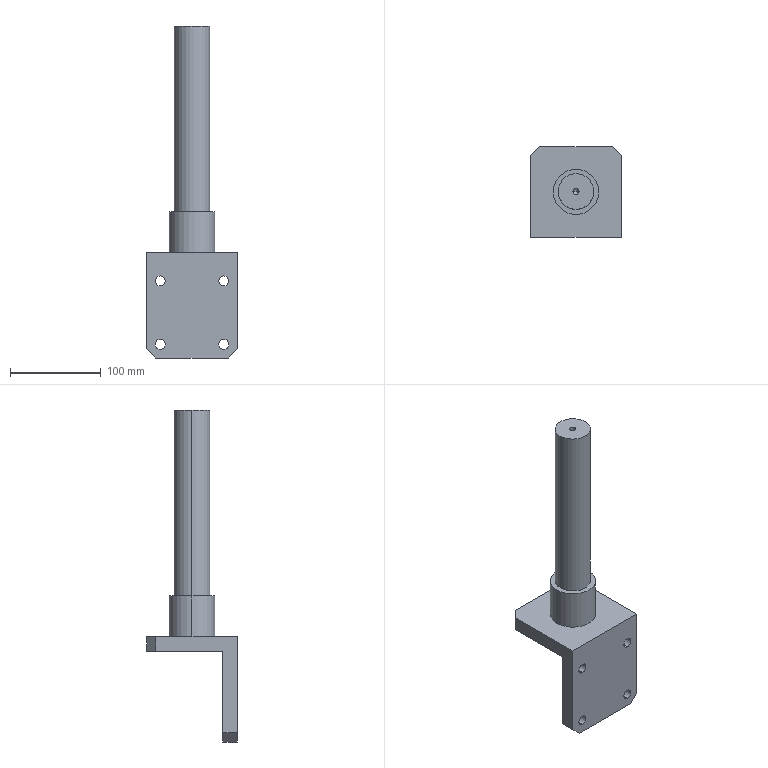Part | SolidWorks | features ICE 3, HoleWzd 2, Chamfer 1, Extrusion 1 | 1 solid | 30 faces | box 100 x 100 x 366 mm | volume 643224 mm3 | cylinder 14 | plane 14 | cone 2 | commonest cylinder face diameters 11 x8 6.8 x2 39 x2 50 x2
STEP:
#1=CARTESIAN_POINT('',(-35.,-50.,-90.5));
#2=VERTEX_POINT('',#1);
#3=CARTESIAN_POINT('',(-35.,-50.,-79.5));
#4=VERTEX_POINT('',#3);
#5=CARTESIAN_POINT('',(-35.,-50.,-85.));
#6=DIRECTION('',(0.,1.,0.));
#7=DIRECTION('',(0.,0.,1.));
#8=AXIS2_PLACEMENT_3D('',#5,#6,#7);
#9=CIRCLE('',#8,5.5);
#10=EDGE_CURVE('',#2,#4,#9,.T.);
#11=ORIENTED_EDGE('',*,*,#10,.F.);
#12=CARTESIAN_POINT('',(-35.,-34.,-90.5));
#13=VERTEX_POINT('',#12);
#14=CARTESIAN_POINT('',(-35.,-34.,-90.5));
#15=DIRECTION('',(0.,1.,0.));
#16=VECTOR('',#15,1000.);
#17=LINE('',#14,#16);
#18=EDGE_CURVE('',#2,#13,#17,.T.);
#19=ORIENTED_EDGE('',*,*,#18,.T.);
#20=CARTESIAN_POINT('',(-35.,-34.,-79.5));
#21=VERTEX_POINT('',#20);
#22=CARTESIAN_POINT('',(-35.,-34.,-85.));
#23=DIRECTION('',(0.,1.,0.));
#24=DIRECTION('',(0.,0.,1.));
#25=AXIS2_PLACEMENT_3D('',#22,#23,#24);
#26=CIRCLE('',#25,5.5);
#27=EDGE_CURVE('',#13,#21,#26,.T.);
#28=ORIENTED_EDGE('',*,*,#27,.T.);
#29=CARTESIAN_POINT('',(-35.,-34.,-79.5));
#30=DIRECTION('',(0.,1.,0.));
#31=VECTOR('',#30,1000.);
#32=LINE('',#29,#31);
#33=EDGE_CURVE('',#4,#21,#32,.T.);
#34=ORIENTED_EDGE('',*,*,#33,.F.);
#35=EDGE_LOOP('',(#11,#19,#28,#34));
#36=FACE_OUTER_BOUND('',#35,.T.);
#37=CARTESIAN_POINT('',(-35.,-34.,-85.));
#38=DIRECTION('',(0.,1.,0.));
#39=DIRECTION('',(0.,0.,1.));
#40=AXIS2_PLACEMENT_3D('',#37,#38,#39);
#41=CYLINDRICAL_SURFACE('',#40,5.5);
#42=ADVANCED_FACE('',(#36),#41,.F.);
#43=CARTESIAN_POINT('',(35.,-50.,-90.5));
#44=VERTEX_POINT('',#43);
#45=CARTESIAN_POINT('',(35.,-50.,-79.5));
#46=VERTEX_POINT('',#45);
#47=CARTESIAN_POINT('',(35.,-50.,-85.));
#48=DIRECTION('',(0.,1.,0.));
#49=DIRECTION('',(0.,0.,1.));
#50=AXIS2_PLACEMENT_3D('',#47,#48,#49);
#51=CIRCLE('',#50,5.5);
#52=EDGE_CURVE('',#44,#46,#51,.T.);
#53=ORIENTED_EDGE('',*,*,#52,.F.);
#54=CARTESIAN_POINT('',(35.,-34.,-90.5));
#55=VERTEX_POINT('',#54);
#56=CARTESIAN_POINT('',(35.,-34.,-90.5));
#57=DIRECTION('',(0.,1.,0.));
#58=VECTOR('',#57,1000.);
#59=LINE('',#56,#58);
#60=EDGE_CURVE('',#44,#55,#59,.T.);
#61=ORIENTED_EDGE('',*,*,#60,.T.);
#62=CARTESIAN_POINT('',(35.,-34.,-79.5));
#63=VERTEX_POINT('',#62);
#64=CARTESIAN_POINT('',(35.,-34.,-85.));
#65=DIRECTION('',(0.,1.,0.));
#66=DIRECTION('',(0.,0.,1.));
#67=AXIS2_PLACEMENT_3D('',#64,#65,#66);
#68=CIRCLE('',#67,5.5);
#69=EDGE_CURVE('',#55,#63,#68,.T.);
#70=ORIENTED_EDGE('',*,*,#69,.T.);
#71=CARTESIAN_POINT('',(35.,-34.,-79.5));
#72=DIRECTION('',(0.,1.,0.));
#73=VECTOR('',#72,1000.);
#74=LINE('',#71,#73);
#75=EDGE_CURVE('',#46,#63,#74,.T.);
#76=ORIENTED_EDGE('',*,*,#75,.F.);
#77=EDGE_LOOP('',(#53,#61,#70,#76));
#78=FACE_OUTER_BOUND('',#77,.T.);
#79=CARTESIAN_POINT('',(35.,-34.,-85.));
#80=DIRECTION('',(0.,1.,0.));
#81=DIRECTION('',(0.,0.,1.));
#82=AXIS2_PLACEMENT_3D('',#79,#80,#81);
#83=CYLINDRICAL_SURFACE('',#82,5.5);
#84=ADVANCED_FACE('',(#78),#83,.F.);
#85=CARTESIAN_POINT('',(35.,-50.,-20.5));
#86=VERTEX_POINT('',#85);
#87=CARTESIAN_POINT('',(35.,-50.,-9.5));
#88=VERTEX_POINT('',#87);
#89=CARTESIAN_POINT('',(35.,-50.,-15.));
#90=DIRECTION('',(0.,1.,0.));
#91=DIRECTION('',(0.,0.,1.));
#92=AXIS2_PLACEMENT_3D('',#89,#90,#91);
#93=CIRCLE('',#92,5.5);
#94=EDGE_CURVE('',#86,#88,#93,.T.);
#95=ORIENTED_EDGE('',*,*,#94,.F.);
#96=CARTESIAN_POINT('',(35.,-34.,-20.5));
#97=VERTEX_POINT('',#96);
#98=CARTESIAN_POINT('',(35.,-34.,-20.5));
#99=DIRECTION('',(0.,1.,0.));
#100=VECTOR('',#99,1000.);
#101=LINE('',#98,#100);
#102=EDGE_CURVE('',#86,#97,#101,.T.);
#103=ORIENTED_EDGE('',*,*,#102,.T.);
#104=CARTESIAN_POINT('',(35.,-34.,-9.5));
#105=VERTEX_POINT('',#104);
#106=CARTESIAN_POINT('',(35.,-34.,-15.));
#107=DIRECTION('',(0.,1.,0.));
#108=DIRECTION('',(0.,0.,1.));
#109=AXIS2_PLACEMENT_3D('',#106,#107,#108);
#110=CIRCLE('',#109,5.5);
#111=EDGE_CURVE('',#97,#105,#110,.T.);
#112=ORIENTED_EDGE('',*,*,#111,.T.);
#113=CARTESIAN_POINT('',(35.,-34.,-9.5));
#114=DIRECTION('',(0.,1.,0.));
#115=VECTOR('',#114,1000.);
#116=LINE('',#113,#115);
#117=EDGE_CURVE('',#88,#105,#116,.T.);
#118=ORIENTED_EDGE('',*,*,#117,.F.);
#119=EDGE_LOOP('',(#95,#103,#112,#118));
#120=FACE_OUTER_BOUND('',#119,.T.);
#121=CARTESIAN_POINT('',(35.,-34.,-15.));
#122=DIRECTION('',(0.,1.,0.));
#123=DIRECTION('',(0.,0.,1.));
#124=AXIS2_PLACEMENT_3D('',#121,#122,#123);
#125=CYLINDRICAL_SURFACE('',#124,5.5);
#126=ADVANCED_FACE('',(#120),#125,.F.);
#127=CARTESIAN_POINT('',(-35.,-50.,-20.5));
#128=VERTEX_POINT('',#127);
#129=CARTESIAN_POINT('',(-35.,-50.,-9.5));
#130=VERTEX_POINT('',#129);
#131=CARTESIAN_POINT('',(-35.,-50.,-15.));
#132=DIRECTION('',(0.,1.,0.));
#133=DIRECTION('',(0.,0.,1.));
#134=AXIS2_PLACEMENT_3D('',#131,#132,#133);
#135=CIRCLE('',#134,5.5);
#136=EDGE_CURVE('',#128,#130,#135,.T.);
#137=ORIENTED_EDGE('',*,*,#136,.F.);
#138=CARTESIAN_POINT('',(-35.,-34.,-20.5));
#139=VERTEX_POINT('',#138);
#140=CARTESIAN_POINT('',(-35.,-34.,-20.5));
#141=DIRECTION('',(0.,1.,0.));
#142=VECTOR('',#141,1000.);
#143=LINE('',#140,#142);
#144=EDGE_CURVE('',#128,#139,#143,.T.);
#145=ORIENTED_EDGE('',*,*,#144,.T.);
#146=CARTESIAN_POINT('',(-35.,-34.,-9.5));
#147=VERTEX_POINT('',#146);
#148=CARTESIAN_POINT('',(-35.,-34.,-15.));
#149=DIRECTION('',(0.,1.,0.));
#150=DIRECTION('',(0.,0.,1.));
#151=AXIS2_PLACEMENT_3D('',#148,#149,#150);
#152=CIRCLE('',#151,5.5);
#153=EDGE_CURVE('',#139,#147,#152,.T.);
#154=ORIENTED_EDGE('',*,*,#153,.T.);
#155=CARTESIAN_POINT('',(-35.,-34.,-9.5));
#156=DIRECTION('',(0.,1.,0.));
#157=VECTOR('',#156,1000.);
#158=LINE('',#155,#157);
#159=EDGE_CURVE('',#130,#147,#158,.T.);
#160=ORIENTED_EDGE('',*,*,#159,.F.);
#161=EDGE_LOOP('',(#137,#145,#154,#160));
#162=FACE_OUTER_BOUND('',#161,.T.);
#163=CARTESIAN_POINT('',(-35.,-34.,-15.));
#164=DIRECTION('',(0.,1.,0.));
#165=DIRECTION('',(0.,0.,1.));
#166=AXIS2_PLACEMENT_3D('',#163,#164,#165);
#167=CYLINDRICAL_SURFACE('',#166,5.5);
#168=ADVANCED_FACE('',(#162),#167,.F.);
#169=CARTESIAN_POINT('',(-3.4,0.,246.25));
#170=VERTEX_POINT('',#169);
#171=CARTESIAN_POINT('',(3.4,0.,246.25));
#172=VERTEX_POINT('',#171);
#173=CARTESIAN_POINT('',(0.,0.,246.25));
#174=DIRECTION('',(0.,0.,1.));
#175=DIRECTION('',(1.,0.,0.));
#176=AXIS2_PLACEMENT_3D('',#173,#174,#175);
#177=CIRCLE('',#176,3.4);
#178=EDGE_CURVE('',#170,#172,#177,.T.);
#179=ORIENTED_EDGE('',*,*,#178,.F.);
#180=CARTESIAN_POINT('',(-3.4,0.,266.));
#181=VERTEX_POINT('',#180);
#182=CARTESIAN_POINT('',(-3.4,0.,266.));
#183=DIRECTION('',(0.,0.,1.));
#184=VECTOR('',#183,1000.);
#185=LINE('',#182,#184);
#186=EDGE_CURVE('',#170,#181,#185,.T.);
#187=ORIENTED_EDGE('',*,*,#186,.T.);
#188=CARTESIAN_POINT('',(3.4,0.,266.));
#189=VERTEX_POINT('',#188);
#190=CARTESIAN_POINT('',(0.,0.,266.));
#191=DIRECTION('',(0.,0.,1.));
#192=DIRECTION('',(1.,0.,0.));
#193=AXIS2_PLACEMENT_3D('',#190,#191,#192);
#194=CIRCLE('',#193,3.4);
#195=EDGE_CURVE('',#181,#189,#194,.T.);
#196=ORIENTED_EDGE('',*,*,#195,.T.);
#197=CARTESIAN_POINT('',(3.4,0.,266.));
#198=DIRECTION('',(0.,0.,1.));
#199=VECTOR('',#198,1000.);
#200=LINE('',#197,#199);
#201=EDGE_CURVE('',#172,#189,#200,.T.);
#202=ORIENTED_EDGE('',*,*,#201,.F.);
#203=EDGE_LOOP('',(#179,#187,#196,#202));
#204=FACE_OUTER_BOUND('',#203,.T.);
#205=CARTESIAN_POINT('',(0.,0.,266.));
#206=DIRECTION('',(0.,0.,1.));
#207=DIRECTION('',(1.,0.,0.));
#208=AXIS2_PLACEMENT_3D('',#205,#206,#207);
#209=CYLINDRICAL_SURFACE('',#208,3.4);
#210=ADVANCED_FACE('',(#204),#209,.F.);
#211=CARTESIAN_POINT('',(0.,0.,244.207));
#212=VERTEX_POINT('',#211);
#213=CARTESIAN_POINT('',(3.4,0.,246.25));
#214=DIRECTION('',(0.8572,0.,0.515));
#215=VECTOR('',#214,1000.);
#216=LINE('',#213,#215);
#217=EDGE_CURVE('',#212,#172,#216,.T.);
#218=ORIENTED_EDGE('',*,*,#217,.F.);
#219=CARTESIAN_POINT('',(-3.4,0.,246.25));
#220=DIRECTION('',(-0.8572,0.,0.515));
#221=VECTOR('',#220,1000.);
#222=LINE('',#219,#221);
#223=EDGE_CURVE('',#212,#170,#222,.T.);
#224=ORIENTED_EDGE('',*,*,#223,.T.);
#225=ORIENTED_EDGE('',*,*,#178,.T.);
#226=EDGE_LOOP('',(#218,#224,#225));
#227=FACE_OUTER_BOUND('',#226,.T.);
#228=CARTESIAN_POINT('',(0.,0.,246.25));
#229=DIRECTION('',(0.,0.,1.));
#230=DIRECTION('',(1.,0.,0.));
#231=AXIS2_PLACEMENT_3D('',#228,#229,#230);
#232=CONICAL_SURFACE('',#231,3.4,1.03);
#233=ADVANCED_FACE('',(#227),#232,.F.);
#234=CARTESIAN_POINT('',(19.5,0.,61.));
#235=VERTEX_POINT('',#234);
#236=CARTESIAN_POINT('',(-19.5,0.,61.));
#237=VERTEX_POINT('',#236);
#238=CARTESIAN_POINT('',(0.,0.,61.));
#239=DIRECTION('',(0.,0.,1.));
#240=DIRECTION('',(1.,0.,0.));
#241=AXIS2_PLACEMENT_3D('',#238,#239,#240);
#242=CIRCLE('',#241,19.5);
#243=EDGE_CURVE('',#235,#237,#242,.T.);
#244=ORIENTED_EDGE('',*,*,#243,.T.);
#245=CARTESIAN_POINT('',(-19.5,0.,266.));
#246=VERTEX_POINT('',#245);
#247=CARTESIAN_POINT('',(-19.5,0.,61.));
#248=DIRECTION('',(0.,0.,1.));
#249=VECTOR('',#248,1000.);
#250=LINE('',#247,#249);
#251=EDGE_CURVE('',#237,#246,#250,.T.);
#252=ORIENTED_EDGE('',*,*,#251,.T.);
#253=CARTESIAN_POINT('',(19.5,0.,266.));
#254=VERTEX_POINT('',#253);
#255=CARTESIAN_POINT('',(0.,0.,266.));
#256=DIRECTION('',(0.,0.,1.));
#257=DIRECTION('',(1.,0.,0.));
#258=AXIS2_PLACEMENT_3D('',#255,#256,#257);
#259=CIRCLE('',#258,19.5);
#260=EDGE_CURVE('',#254,#246,#259,.T.);
#261=ORIENTED_EDGE('',*,*,#260,.F.);
#262=CARTESIAN_POINT('',(19.5,0.,61.));
#263=DIRECTION('',(0.,0.,1.));
#264=VECTOR('',#263,1000.);
#265=LINE('',#262,#264);
#266=EDGE_CURVE('',#235,#254,#265,.T.);
#267=ORIENTED_EDGE('',*,*,#266,.F.);
#268=EDGE_LOOP('',(#244,#252,#261,#267));
#269=FACE_OUTER_BOUND('',#268,.T.);
#270=CARTESIAN_POINT('',(0.,0.,61.));
#271=DIRECTION('',(0.,0.,1.));
#272=DIRECTION('',(1.,0.,0.));
#273=AXIS2_PLACEMENT_3D('',#270,#271,#272);
#274=CYLINDRICAL_SURFACE('',#273,19.5);
#275=ADVANCED_FACE('',(#269),#274,.T.);
#276=CARTESIAN_POINT('',(25.,0.,61.));
#277=VERTEX_POINT('',#276);
#278=CARTESIAN_POINT('',(-25.,0.,61.));
#279=VERTEX_POINT('',#278);
#280=CARTESIAN_POINT('',(0.,0.,61.));
#281=DIRECTION('',(0.,0.,1.));
#282=DIRECTION('',(1.,0.,0.));
#283=AXIS2_PLACEMENT_3D('',#280,#281,#282);
#284=CIRCLE('',#283,25.);
#285=EDGE_CURVE('',#277,#279,#284,.T.);
#286=ORIENTED_EDGE('',*,*,#285,.F.);
#287=CARTESIAN_POINT('',(25.,0.,16.));
#288=VERTEX_POINT('',#287);
#289=CARTESIAN_POINT('',(25.,0.,266.));
#290=DIRECTION('',(0.,0.,-1.));
#291=VECTOR('',#290,1000.);
#292=LINE('',#289,#291);
#293=EDGE_CURVE('',#277,#288,#292,.T.);
#294=ORIENTED_EDGE('',*,*,#293,.T.);
#295=CARTESIAN_POINT('',(-25.,0.,16.));
#296=VERTEX_POINT('',#295);
#297=CARTESIAN_POINT('',(0.,0.,16.));
#298=DIRECTION('',(0.,0.,1.));
#299=DIRECTION('',(1.,0.,0.));
#300=AXIS2_PLACEMENT_3D('',#297,#298,#299);
#301=CIRCLE('',#300,25.);
#302=EDGE_CURVE('',#288,#296,#301,.T.);
#303=ORIENTED_EDGE('',*,*,#302,.T.);
#304=CARTESIAN_POINT('',(-25.,0.,266.));
#305=DIRECTION('',(0.,0.,-1.));
#306=VECTOR('',#305,1000.);
#307=LINE('',#304,#306);
#308=EDGE_CURVE('',#279,#296,#307,.T.);
#309=ORIENTED_EDGE('',*,*,#308,.F.);
#310=EDGE_LOOP('',(#286,#294,#303,#309));
#311=FACE_OUTER_BOUND('',#310,.T.);
#312=CARTESIAN_POINT('',(0.,0.,266.));
#313=DIRECTION('',(0.,0.,-1.));
#314=DIRECTION('',(-1.,0.,0.));
#315=AXIS2_PLACEMENT_3D('',#312,#313,#314);
#316=CYLINDRICAL_SURFACE('',#315,25.);
#317=ADVANCED_FACE('',(#311),#316,.T.);
#318=CARTESIAN_POINT('',(-35.,-34.,-85.));
#319=DIRECTION('',(0.,1.,0.));
#320=DIRECTION('',(0.,0.,1.));
#321=AXIS2_PLACEMENT_3D('',#318,#319,#320);
#322=CIRCLE('',#321,5.5);
#323=EDGE_CURVE('',#21,#13,#322,.T.);
#324=ORIENTED_EDGE('',*,*,#323,.F.);
#325=ORIENTED_EDGE('',*,*,#27,.F.);
#326=EDGE_LOOP('',(#324,#325));
#327=FACE_BOUND('',#326,.T.);
#328=CARTESIAN_POINT('',(35.,-34.,-85.));
#329=DIRECTION('',(0.,1.,0.));
#330=DIRECTION('',(0.,0.,1.));
#331=AXIS2_PLACEMENT_3D('',#328,#329,#330);
#332=CIRCLE('',#331,5.5);
#333=EDGE_CURVE('',#63,#55,#332,.T.);
#334=ORIENTED_EDGE('',*,*,#333,.F.);
#335=ORIENTED_EDGE('',*,*,#69,.F.);
#336=EDGE_LOOP('',(#334,#335));
#337=FACE_BOUND('',#336,.T.);
#338=CARTESIAN_POINT('',(35.,-34.,-15.));
#339=DIRECTION('',(0.,1.,0.));
#340=DIRECTION('',(0.,0.,1.));
#341=AXIS2_PLACEMENT_3D('',#338,#339,#340);
#342=CIRCLE('',#341,5.5);
#343=EDGE_CURVE('',#105,#97,#342,.T.);
#344=ORIENTED_EDGE('',*,*,#343,.F.);
#345=ORIENTED_EDGE('',*,*,#111,.F.);
#346=EDGE_LOOP('',(#344,#345));
#347=FACE_BOUND('',#346,.T.);
#348=CARTESIAN_POINT('',(-40.,-34.,-100.));
#349=VERTEX_POINT('',#348);
#350=CARTESIAN_POINT('',(40.,-34.,-100.));
#351=VERTEX_POINT('',#350);
#352=CARTESIAN_POINT('',(-50.,-34.,-100.));
#353=DIRECTION('',(1.,0.,0.));
#354=VECTOR('',#353,1000.);
#355=LINE('',#352,#354);
#356=EDGE_CURVE('',#349,#351,#355,.T.);
#357=ORIENTED_EDGE('',*,*,#356,.F.);
#358=CARTESIAN_POINT('',(-50.,-34.,-90.));
#359=VERTEX_POINT('',#358);
#360=CARTESIAN_POINT('',(-40.,-34.,-100.));
#361=DIRECTION('',(-0.7071,0.,0.7071));
#362=VECTOR('',#361,1000.);
#363=LINE('',#360,#362);
#364=EDGE_CURVE('',#349,#359,#363,.T.);
#365=ORIENTED_EDGE('',*,*,#364,.T.);
#366=CARTESIAN_POINT('',(-50.,-34.,0.));
#367=VERTEX_POINT('',#366);
#368=CARTESIAN_POINT('',(-50.,-34.,-100.));
#369=DIRECTION('',(0.,0.,1.));
#370=VECTOR('',#369,1000.);
#371=LINE('',#368,#370);
#372=EDGE_CURVE('',#359,#367,#371,.T.);
#373=ORIENTED_EDGE('',*,*,#372,.T.);
#374=CARTESIAN_POINT('',(50.,-34.,0.));
#375=VERTEX_POINT('',#374);
#376=CARTESIAN_POINT('',(-50.,-34.,0.));
#377=DIRECTION('',(1.,0.,0.));
#378=VECTOR('',#377,1000.);
#379=LINE('',#376,#378);
#380=EDGE_CURVE('',#367,#375,#379,.T.);
#381=ORIENTED_EDGE('',*,*,#380,.T.);
#382=CARTESIAN_POINT('',(50.,-34.,-90.));
#383=VERTEX_POINT('',#382);
#384=CARTESIAN_POINT('',(50.,-34.,-100.));
#385=DIRECTION('',(0.,0.,1.));
#386=VECTOR('',#385,1000.);
#387=LINE('',#384,#386);
#388=EDGE_CURVE('',#383,#375,#387,.T.);
#389=ORIENTED_EDGE('',*,*,#388,.F.);
#390=CARTESIAN_POINT('',(40.,-34.,-100.));
#391=DIRECTION('',(-0.7071,0.,-0.7071));
#392=VECTOR('',#391,1000.);
#393=LINE('',#390,#392);
#394=EDGE_CURVE('',#383,#351,#393,.T.);
#395=ORIENTED_EDGE('',*,*,#394,.T.);
#396=EDGE_LOOP('',(#357,#365,#373,#381,#389,#395));
#397=FACE_OUTER_BOUND('',#396,.T.);
#398=CARTESIAN_POINT('',(-35.,-34.,-15.));
#399=DIRECTION('',(0.,1.,0.));
#400=DIRECTION('',(0.,0.,1.));
#401=AXIS2_PLACEMENT_3D('',#398,#399,#400);
#402=CIRCLE('',#401,5.5);
#403=EDGE_CURVE('',#147,#139,#402,.T.);
#404=ORIENTED_EDGE('',*,*,#403,.F.);
#405=ORIENTED_EDGE('',*,*,#153,.F.);
#406=EDGE_LOOP('',(#404,#405));
#407=FACE_BOUND('',#406,.T.);
#408=CARTESIAN_POINT('',(-50.,-34.,-100.));
#409=DIRECTION('',(0.,-1.,0.));
#410=DIRECTION('',(1.,0.,0.));
#411=AXIS2_PLACEMENT_3D('',#408,#409,#410);
#412=PLANE('',#411);
#413=ADVANCED_FACE('',(#327,#337,#347,#397,#407),#412,.F.);
#414=ORIENTED_EDGE('',*,*,#293,.F.);
#415=CARTESIAN_POINT('',(0.,0.,61.));
#416=DIRECTION('',(0.,0.,1.));
#417=DIRECTION('',(1.,0.,0.));
#418=AXIS2_PLACEMENT_3D('',#415,#416,#417);
#419=CIRCLE('',#418,25.);
#420=EDGE_CURVE('',#279,#277,#419,.T.);
#421=ORIENTED_EDGE('',*,*,#420,.F.);
#422=ORIENTED_EDGE('',*,*,#308,.T.);
#423=CARTESIAN_POINT('',(0.,0.,16.));
#424=DIRECTION('',(0.,0.,1.));
#425=DIRECTION('',(1.,0.,0.));
#426=AXIS2_PLACEMENT_3D('',#423,#424,#425);
#427=CIRCLE('',#426,25.);
#428=EDGE_CURVE('',#296,#288,#427,.T.);
#429=ORIENTED_EDGE('',*,*,#428,.T.);
#430=EDGE_LOOP('',(#414,#421,#422,#429));
#431=FACE_OUTER_BOUND('',#430,.T.);
#432=CARTESIAN_POINT('',(0.,0.,266.));
#433=DIRECTION('',(0.,0.,-1.));
#434=DIRECTION('',(-1.,0.,0.));
#435=AXIS2_PLACEMENT_3D('',#432,#433,#434);
#436=CYLINDRICAL_SURFACE('',#435,25.);
#437=ADVANCED_FACE('',(#431),#436,.T.);
#438=CARTESIAN_POINT('',(50.,-50.,16.));
#439=VERTEX_POINT('',#438);
#440=CARTESIAN_POINT('',(50.,-50.,-90.));
#441=VERTEX_POINT('',#440);
#442=CARTESIAN_POINT('',(50.,-50.,16.));
#443=DIRECTION('',(0.,0.,-1.));
#444=VECTOR('',#443,1000.);
#445=LINE('',#442,#444);
#446=EDGE_CURVE('',#439,#441,#445,.T.);
#447=ORIENTED_EDGE('',*,*,#446,.T.);
#448=CARTESIAN_POINT('',(50.,-34.,-90.));
#449=DIRECTION('',(0.,1.,0.));
#450=VECTOR('',#449,1000.);
#451=LINE('',#448,#450);
#452=EDGE_CURVE('',#441,#383,#451,.T.);
#453=ORIENTED_EDGE('',*,*,#452,.T.);
#454=ORIENTED_EDGE('',*,*,#388,.T.);
#455=CARTESIAN_POINT('',(50.,40.,0.));
#456=VERTEX_POINT('',#455);
#457=CARTESIAN_POINT('',(50.,-50.,0.));
#458=DIRECTION('',(0.,1.,0.));
#459=VECTOR('',#458,1000.);
#460=LINE('',#457,#459);
#461=EDGE_CURVE('',#375,#456,#460,.T.);
#462=ORIENTED_EDGE('',*,*,#461,.T.);
#463=CARTESIAN_POINT('',(50.,40.,16.));
#464=VERTEX_POINT('',#463);
#465=CARTESIAN_POINT('',(50.,40.,16.));
#466=DIRECTION('',(0.,0.,1.));
#467=VECTOR('',#466,1000.);
#468=LINE('',#465,#467);
#469=EDGE_CURVE('',#456,#464,#468,.T.);
#470=ORIENTED_EDGE('',*,*,#469,.T.);
#471=CARTESIAN_POINT('',(50.,-50.,16.));
#472=DIRECTION('',(0.,1.,0.));
#473=VECTOR('',#472,1000.);
#474=LINE('',#471,#473);
#475=EDGE_CURVE('',#439,#464,#474,.T.);
#476=ORIENTED_EDGE('',*,*,#475,.F.);
#477=EDGE_LOOP('',(#447,#453,#454,#462,#470,#476));
#478=FACE_OUTER_BOUND('',#477,.T.);
#479=CARTESIAN_POINT('',(50.,-50.,16.));
#480=DIRECTION('',(-1.,0.,0.));
#481=DIRECTION('',(0.,0.,1.));
#482=AXIS2_PLACEMENT_3D('',#479,#480,#481);
#483=PLANE('',#482);
#484=ADVANCED_FACE('',(#478),#483,.F.);
#485=CARTESIAN_POINT('',(40.,50.,16.));
#486=VERTEX_POINT('',#485);
#487=CARTESIAN_POINT('',(-40.,50.,16.));
#488=VERTEX_POINT('',#487);
#489=CARTESIAN_POINT('',(-50.,50.,16.));
#490=DIRECTION('',(-1.,0.,0.));
#491=VECTOR('',#490,1000.);
#492=LINE('',#489,#491);
#493=EDGE_CURVE('',#486,#488,#492,.T.);
#494=ORIENTED_EDGE('',*,*,#493,.F.);
#495=CARTESIAN_POINT('',(40.,50.,0.));
#496=VERTEX_POINT('',#495);
#497=CARTESIAN_POINT('',(40.,50.,16.));
#498=DIRECTION('',(0.,0.,-1.));
#499=VECTOR('',#498,1000.);
#500=LINE('',#497,#499);
#501=EDGE_CURVE('',#486,#496,#500,.T.);
#502=ORIENTED_EDGE('',*,*,#501,.T.);
#503=CARTESIAN_POINT('',(-40.,50.,0.));
#504=VERTEX_POINT('',#503);
#505=CARTESIAN_POINT('',(-50.,50.,0.));
#506=DIRECTION('',(-1.,0.,0.));
#507=VECTOR('',#506,1000.);
#508=LINE('',#505,#507);
#509=EDGE_CURVE('',#496,#504,#508,.T.);
#510=ORIENTED_EDGE('',*,*,#509,.T.);
#511=CARTESIAN_POINT('',(-40.,50.,16.));
#512=DIRECTION('',(0.,0.,1.));
#513=VECTOR('',#512,1000.);
#514=LINE('',#511,#513);
#515=EDGE_CURVE('',#504,#488,#514,.T.);
#516=ORIENTED_EDGE('',*,*,#515,.T.);
#517=EDGE_LOOP('',(#494,#502,#510,#516));
#518=FACE_OUTER_BOUND('',#517,.T.);
#519=CARTESIAN_POINT('',(-50.,50.,16.));
#520=DIRECTION('',(0.,-1.,0.));
#521=DIRECTION('',(0.,0.,-1.));
#522=AXIS2_PLACEMENT_3D('',#519,#520,#521);
#523=PLANE('',#522);
#524=ADVANCED_FACE('',(#518),#523,.F.);
#525=ORIENTED_EDGE('',*,*,#372,.F.);
#526=CARTESIAN_POINT('',(-50.,-50.,-90.));
#527=VERTEX_POINT('',#526);
#528=CARTESIAN_POINT('',(-50.,-50.,-90.));
#529=DIRECTION('',(0.,-1.,0.));
#530=VECTOR('',#529,1000.);
#531=LINE('',#528,#530);
#532=EDGE_CURVE('',#359,#527,#531,.T.);
#533=ORIENTED_EDGE('',*,*,#532,.T.);
#534=CARTESIAN_POINT('',(-50.,-50.,16.));
#535=VERTEX_POINT('',#534);
#536=CARTESIAN_POINT('',(-50.,-50.,16.));
#537=DIRECTION('',(0.,0.,-1.));
#538=VECTOR('',#537,1000.);
#539=LINE('',#536,#538);
#540=EDGE_CURVE('',#535,#527,#539,.T.);
#541=ORIENTED_EDGE('',*,*,#540,.F.);
#542=CARTESIAN_POINT('',(-50.,40.,16.));
#543=VERTEX_POINT('',#542);
#544=CARTESIAN_POINT('',(-50.,-50.,16.));
#545=DIRECTION('',(0.,-1.,0.));
#546=VECTOR('',#545,1000.);
#547=LINE('',#544,#546);
#548=EDGE_CURVE('',#543,#535,#547,.T.);
#549=ORIENTED_EDGE('',*,*,#548,.F.);
#550=CARTESIAN_POINT('',(-50.,40.,0.));
#551=VERTEX_POINT('',#550);
#552=CARTESIAN_POINT('',(-50.,40.,16.));
#553=DIRECTION('',(0.,0.,-1.));
#554=VECTOR('',#553,1000.);
#555=LINE('',#552,#554);
#556=EDGE_CURVE('',#543,#551,#555,.T.);
#557=ORIENTED_EDGE('',*,*,#556,.T.);
#558=CARTESIAN_POINT('',(-50.,-50.,0.));
#559=DIRECTION('',(0.,-1.,0.));
#560=VECTOR('',#559,1000.);
#561=LINE('',#558,#560);
#562=EDGE_CURVE('',#551,#367,#561,.T.);
#563=ORIENTED_EDGE('',*,*,#562,.T.);
#564=EDGE_LOOP('',(#525,#533,#541,#549,#557,#563));
#565=FACE_OUTER_BOUND('',#564,.T.);
#566=CARTESIAN_POINT('',(-50.,-50.,16.));
#567=DIRECTION('',(1.,0.,0.));
#568=DIRECTION('',(0.,0.,-1.));
#569=AXIS2_PLACEMENT_3D('',#566,#567,#568);
#570=PLANE('',#569);
#571=ADVANCED_FACE('',(#565),#570,.F.);
#572=CARTESIAN_POINT('',(-35.,-50.,-85.));
#573=DIRECTION('',(0.,1.,0.));
#574=DIRECTION('',(0.,0.,1.));
#575=AXIS2_PLACEMENT_3D('',#572,#573,#574);
#576=CIRCLE('',#575,5.5);
#577=EDGE_CURVE('',#4,#2,#576,.T.);
#578=ORIENTED_EDGE('',*,*,#577,.T.);
#579=ORIENTED_EDGE('',*,*,#10,.T.);
#580=EDGE_LOOP('',(#578,#579));
#581=FACE_BOUND('',#580,.T.);
#582=CARTESIAN_POINT('',(35.,-50.,-85.));
#583=DIRECTION('',(0.,1.,0.));
#584=DIRECTION('',(0.,0.,1.));
#585=AXIS2_PLACEMENT_3D('',#582,#583,#584);
#586=CIRCLE('',#585,5.5);
#587=EDGE_CURVE('',#46,#44,#586,.T.);
#588=ORIENTED_EDGE('',*,*,#587,.T.);
#589=ORIENTED_EDGE('',*,*,#52,.T.);
#590=EDGE_LOOP('',(#588,#589));
#591=FACE_BOUND('',#590,.T.);
#592=CARTESIAN_POINT('',(35.,-50.,-15.));
#593=DIRECTION('',(0.,1.,0.));
#594=DIRECTION('',(0.,0.,1.));
#595=AXIS2_PLACEMENT_3D('',#592,#593,#594);
#596=CIRCLE('',#595,5.5);
#597=EDGE_CURVE('',#88,#86,#596,.T.);
#598=ORIENTED_EDGE('',*,*,#597,.T.);
#599=ORIENTED_EDGE('',*,*,#94,.T.);
#600=EDGE_LOOP('',(#598,#599));
#601=FACE_BOUND('',#600,.T.);
#602=CARTESIAN_POINT('',(-35.,-50.,-15.));
#603=DIRECTION('',(0.,1.,0.));
#604=DIRECTION('',(0.,0.,1.));
#605=AXIS2_PLACEMENT_3D('',#602,#603,#604);
#606=CIRCLE('',#605,5.5);
#607=EDGE_CURVE('',#130,#128,#606,.T.);
#608=ORIENTED_EDGE('',*,*,#607,.T.);
#609=ORIENTED_EDGE('',*,*,#136,.T.);
#610=EDGE_LOOP('',(#608,#609));
#611=FACE_BOUND('',#610,.T.);
#612=ORIENTED_EDGE('',*,*,#540,.T.);
#613=CARTESIAN_POINT('',(-40.,-50.,-100.));
#614=VERTEX_POINT('',#613);
#615=CARTESIAN_POINT('',(-40.,-50.,-100.));
#616=DIRECTION('',(0.7071,0.,-0.7071));
#617=VECTOR('',#616,1000.);
#618=LINE('',#615,#617);
#619=EDGE_CURVE('',#527,#614,#618,.T.);
#620=ORIENTED_EDGE('',*,*,#619,.T.);
#621=CARTESIAN_POINT('',(40.,-50.,-100.));
#622=VERTEX_POINT('',#621);
#623=CARTESIAN_POINT('',(-50.,-50.,-100.));
#624=DIRECTION('',(-1.,0.,0.));
#625=VECTOR('',#624,1000.);
#626=LINE('',#623,#625);
#627=EDGE_CURVE('',#622,#614,#626,.T.);
#628=ORIENTED_EDGE('',*,*,#627,.F.);
#629=CARTESIAN_POINT('',(40.,-50.,-100.));
#630=DIRECTION('',(0.7071,0.,0.7071));
#631=VECTOR('',#630,1000.);
#632=LINE('',#629,#631);
#633=EDGE_CURVE('',#622,#441,#632,.T.);
#634=ORIENTED_EDGE('',*,*,#633,.T.);
#635=ORIENTED_EDGE('',*,*,#446,.F.);
#636=CARTESIAN_POINT('',(-50.,-50.,16.));
#637=DIRECTION('',(1.,0.,0.));
#638=VECTOR('',#637,1000.);
#639=LINE('',#636,#638);
#640=EDGE_CURVE('',#535,#439,#639,.T.);
#641=ORIENTED_EDGE('',*,*,#640,.F.);
#642=EDGE_LOOP('',(#612,#620,#628,#634,#635,#641));
#643=FACE_OUTER_BOUND('',#642,.T.);
#644=CARTESIAN_POINT('',(-50.,-50.,16.));
#645=DIRECTION('',(0.,1.,0.));
#646=DIRECTION('',(0.,0.,1.));
#647=AXIS2_PLACEMENT_3D('',#644,#645,#646);
#648=PLANE('',#647);
#649=ADVANCED_FACE('',(#581,#591,#601,#611,#643),#648,.F.);
#650=ORIENTED_EDGE('',*,*,#428,.F.);
#651=ORIENTED_EDGE('',*,*,#302,.F.);
#652=EDGE_LOOP('',(#650,#651));
#653=FACE_BOUND('',#652,.T.);
#654=ORIENTED_EDGE('',*,*,#475,.T.);
#655=CARTESIAN_POINT('',(40.,50.,16.));
#656=DIRECTION('',(-0.7071,0.7071,0.));
#657=VECTOR('',#656,1000.);
#658=LINE('',#655,#657);
#659=EDGE_CURVE('',#464,#486,#658,.T.);
#660=ORIENTED_EDGE('',*,*,#659,.T.);
#661=ORIENTED_EDGE('',*,*,#493,.T.);
#662=CARTESIAN_POINT('',(-50.,40.,16.));
#663=DIRECTION('',(-0.7071,-0.7071,0.));
#664=VECTOR('',#663,1000.);
#665=LINE('',#662,#664);
#666=EDGE_CURVE('',#488,#543,#665,.T.);
#667=ORIENTED_EDGE('',*,*,#666,.T.);
#668=ORIENTED_EDGE('',*,*,#548,.T.);
#669=ORIENTED_EDGE('',*,*,#640,.T.);
#670=EDGE_LOOP('',(#654,#660,#661,#667,#668,#669));
#671=FACE_OUTER_BOUND('',#670,.T.);
#672=CARTESIAN_POINT('',(0.,0.,16.));
#673=DIRECTION('',(0.,0.,-1.));
#674=DIRECTION('',(-1.,0.,0.));
#675=AXIS2_PLACEMENT_3D('',#672,#673,#674);
#676=PLANE('',#675);
#677=ADVANCED_FACE('',(#653,#671),#676,.F.);
#678=ORIENTED_EDGE('',*,*,#509,.F.);
#679=CARTESIAN_POINT('',(45.,45.,0.));
#680=DIRECTION('',(0.7071,-0.7071,0.));
#681=VECTOR('',#680,1000.);
#682=LINE('',#679,#681);
#683=EDGE_CURVE('',#496,#456,#682,.T.);
#684=ORIENTED_EDGE('',*,*,#683,.T.);
#685=ORIENTED_EDGE('',*,*,#461,.F.);
#686=ORIENTED_EDGE('',*,*,#380,.F.);
#687=ORIENTED_EDGE('',*,*,#562,.F.);
#688=CARTESIAN_POINT('',(-45.,45.,0.));
#689=DIRECTION('',(0.7071,0.7071,0.));
#690=VECTOR('',#689,1000.);
#691=LINE('',#688,#690);
#692=EDGE_CURVE('',#551,#504,#691,.T.);
#693=ORIENTED_EDGE('',*,*,#692,.T.);
#694=EDGE_LOOP('',(#678,#684,#685,#686,#687,#693));
#695=FACE_OUTER_BOUND('',#694,.T.);
#696=CARTESIAN_POINT('',(0.,0.,0.));
#697=DIRECTION('',(0.,0.,-1.));
#698=DIRECTION('',(-1.,0.,0.));
#699=AXIS2_PLACEMENT_3D('',#696,#697,#698);
#700=PLANE('',#699);
#701=ADVANCED_FACE('',(#695),#700,.T.);
#702=ORIENTED_EDGE('',*,*,#243,.F.);
#703=CARTESIAN_POINT('',(0.,0.,61.));
#704=DIRECTION('',(0.,0.,1.));
#705=DIRECTION('',(1.,0.,0.));
#706=AXIS2_PLACEMENT_3D('',#703,#704,#705);
#707=CIRCLE('',#706,19.5);
#708=EDGE_CURVE('',#237,#235,#707,.T.);
#709=ORIENTED_EDGE('',*,*,#708,.F.);
#710=EDGE_LOOP('',(#702,#709));
#711=FACE_BOUND('',#710,.T.);
#712=ORIENTED_EDGE('',*,*,#420,.T.);
#713=ORIENTED_EDGE('',*,*,#285,.T.);
#714=EDGE_LOOP('',(#712,#713));
#715=FACE_OUTER_BOUND('',#714,.T.);
#716=CARTESIAN_POINT('',(0.,0.,61.));
#717=DIRECTION('',(0.,0.,1.));
#718=DIRECTION('',(1.,0.,0.));
#719=AXIS2_PLACEMENT_3D('',#716,#717,#718);
#720=PLANE('',#719);
#721=ADVANCED_FACE('',(#711,#715),#720,.T.);
#722=ORIENTED_EDGE('',*,*,#251,.F.);
#723=ORIENTED_EDGE('',*,*,#708,.T.);
#724=ORIENTED_EDGE('',*,*,#266,.T.);
#725=CARTESIAN_POINT('',(0.,0.,266.));
#726=DIRECTION('',(0.,0.,1.));
#727=DIRECTION('',(1.,0.,0.));
#728=AXIS2_PLACEMENT_3D('',#725,#726,#727);
#729=CIRCLE('',#728,19.5);
#730=EDGE_CURVE('',#246,#254,#729,.T.);
#731=ORIENTED_EDGE('',*,*,#730,.F.);
#732=EDGE_LOOP('',(#722,#723,#724,#731));
#733=FACE_OUTER_BOUND('',#732,.T.);
#734=CARTESIAN_POINT('',(0.,0.,61.));
#735=DIRECTION('',(0.,0.,1.));
#736=DIRECTION('',(1.,0.,0.));
#737=AXIS2_PLACEMENT_3D('',#734,#735,#736);
#738=CYLINDRICAL_SURFACE('',#737,19.5);
#739=ADVANCED_FACE('',(#733),#738,.T.);
#740=CARTESIAN_POINT('',(0.,0.,266.));
#741=DIRECTION('',(0.,0.,1.));
#742=DIRECTION('',(1.,0.,0.));
#743=AXIS2_PLACEMENT_3D('',#740,#741,#742);
#744=CIRCLE('',#743,3.4);
#745=EDGE_CURVE('',#189,#181,#744,.T.);
#746=ORIENTED_EDGE('',*,*,#745,.F.);
#747=ORIENTED_EDGE('',*,*,#195,.F.);
#748=EDGE_LOOP('',(#746,#747));
#749=FACE_BOUND('',#748,.T.);
#750=ORIENTED_EDGE('',*,*,#260,.T.);
#751=ORIENTED_EDGE('',*,*,#730,.T.);
#752=EDGE_LOOP('',(#750,#751));
#753=FACE_OUTER_BOUND('',#752,.T.);
#754=CARTESIAN_POINT('',(0.,0.,266.));
#755=DIRECTION('',(0.,0.,1.));
#756=DIRECTION('',(1.,0.,0.));
#757=AXIS2_PLACEMENT_3D('',#754,#755,#756);
#758=PLANE('',#757);
#759=ADVANCED_FACE('',(#749,#753),#758,.T.);
#760=ORIENTED_EDGE('',*,*,#627,.T.);
#761=CARTESIAN_POINT('',(-40.,-34.,-100.));
#762=DIRECTION('',(0.,1.,0.));
#763=VECTOR('',#762,1000.);
#764=LINE('',#761,#763);
#765=EDGE_CURVE('',#614,#349,#764,.T.);
#766=ORIENTED_EDGE('',*,*,#765,.T.);
#767=ORIENTED_EDGE('',*,*,#356,.T.);
#768=CARTESIAN_POINT('',(40.,-50.,-100.));
#769=DIRECTION('',(0.,-1.,0.));
#770=VECTOR('',#769,1000.);
#771=LINE('',#768,#770);
#772=EDGE_CURVE('',#351,#622,#771,.T.);
#773=ORIENTED_EDGE('',*,*,#772,.T.);
#774=EDGE_LOOP('',(#760,#766,#767,#773));
#775=FACE_OUTER_BOUND('',#774,.T.);
#776=CARTESIAN_POINT('',(0.,0.,-100.));
#777=DIRECTION('',(0.,0.,-1.));
#778=DIRECTION('',(-1.,0.,0.));
#779=AXIS2_PLACEMENT_3D('',#776,#777,#778);
#780=PLANE('',#779);
#781=ADVANCED_FACE('',(#775),#780,.T.);
#782=ORIENTED_EDGE('',*,*,#223,.F.);
#783=ORIENTED_EDGE('',*,*,#217,.T.);
#784=CARTESIAN_POINT('',(0.,0.,246.25));
#785=DIRECTION('',(0.,0.,1.));
#786=DIRECTION('',(1.,0.,0.));
#787=AXIS2_PLACEMENT_3D('',#784,#785,#786);
#788=CIRCLE('',#787,3.4);
#789=EDGE_CURVE('',#172,#170,#788,.T.);
#790=ORIENTED_EDGE('',*,*,#789,.T.);
#791=EDGE_LOOP('',(#782,#783,#790));
#792=FACE_OUTER_BOUND('',#791,.T.);
#793=CARTESIAN_POINT('',(0.,0.,246.25));
#794=DIRECTION('',(0.,0.,1.));
#795=DIRECTION('',(1.,0.,0.));
#796=AXIS2_PLACEMENT_3D('',#793,#794,#795);
#797=CONICAL_SURFACE('',#796,3.4,1.03);
#798=ADVANCED_FACE('',(#792),#797,.F.);
#799=ORIENTED_EDGE('',*,*,#186,.F.);
#800=ORIENTED_EDGE('',*,*,#789,.F.);
#801=ORIENTED_EDGE('',*,*,#201,.T.);
#802=ORIENTED_EDGE('',*,*,#745,.T.);
#803=EDGE_LOOP('',(#799,#800,#801,#802));
#804=FACE_OUTER_BOUND('',#803,.T.);
#805=CARTESIAN_POINT('',(0.,0.,266.));
#806=DIRECTION('',(0.,0.,1.));
#807=DIRECTION('',(1.,0.,0.));
#808=AXIS2_PLACEMENT_3D('',#805,#806,#807);
#809=CYLINDRICAL_SURFACE('',#808,3.4);
#810=ADVANCED_FACE('',(#804),#809,.F.);
#811=ORIENTED_EDGE('',*,*,#144,.F.);
#812=ORIENTED_EDGE('',*,*,#607,.F.);
#813=ORIENTED_EDGE('',*,*,#159,.T.);
#814=ORIENTED_EDGE('',*,*,#403,.T.);
#815=EDGE_LOOP('',(#811,#812,#813,#814));
#816=FACE_OUTER_BOUND('',#815,.T.);
#817=CARTESIAN_POINT('',(-35.,-34.,-15.));
#818=DIRECTION('',(0.,1.,0.));
#819=DIRECTION('',(0.,0.,1.));
#820=AXIS2_PLACEMENT_3D('',#817,#818,#819);
#821=CYLINDRICAL_SURFACE('',#820,5.5);
#822=ADVANCED_FACE('',(#816),#821,.F.);
#823=ORIENTED_EDGE('',*,*,#102,.F.);
#824=ORIENTED_EDGE('',*,*,#597,.F.);
#825=ORIENTED_EDGE('',*,*,#117,.T.);
#826=ORIENTED_EDGE('',*,*,#343,.T.);
#827=EDGE_LOOP('',(#823,#824,#825,#826));
#828=FACE_OUTER_BOUND('',#827,.T.);
#829=CARTESIAN_POINT('',(35.,-34.,-15.));
#830=DIRECTION('',(0.,1.,0.));
#831=DIRECTION('',(0.,0.,1.));
#832=AXIS2_PLACEMENT_3D('',#829,#830,#831);
#833=CYLINDRICAL_SURFACE('',#832,5.5);
#834=ADVANCED_FACE('',(#828),#833,.F.);
#835=ORIENTED_EDGE('',*,*,#60,.F.);
#836=ORIENTED_EDGE('',*,*,#587,.F.);
#837=ORIENTED_EDGE('',*,*,#75,.T.);
#838=ORIENTED_EDGE('',*,*,#333,.T.);
#839=EDGE_LOOP('',(#835,#836,#837,#838));
#840=FACE_OUTER_BOUND('',#839,.T.);
#841=CARTESIAN_POINT('',(35.,-34.,-85.));
#842=DIRECTION('',(0.,1.,0.));
#843=DIRECTION('',(0.,0.,1.));
#844=AXIS2_PLACEMENT_3D('',#841,#842,#843);
#845=CYLINDRICAL_SURFACE('',#844,5.5);
#846=ADVANCED_FACE('',(#840),#845,.F.);
#847=ORIENTED_EDGE('',*,*,#18,.F.);
#848=ORIENTED_EDGE('',*,*,#577,.F.);
#849=ORIENTED_EDGE('',*,*,#33,.T.);
#850=ORIENTED_EDGE('',*,*,#323,.T.);
#851=EDGE_LOOP('',(#847,#848,#849,#850));
#852=FACE_OUTER_BOUND('',#851,.T.);
#853=CARTESIAN_POINT('',(-35.,-34.,-85.));
#854=DIRECTION('',(0.,1.,0.));
#855=DIRECTION('',(0.,0.,1.));
#856=AXIS2_PLACEMENT_3D('',#853,#854,#855);
#857=CYLINDRICAL_SURFACE('',#856,5.5);
#858=ADVANCED_FACE('',(#852),#857,.F.);
#859=ORIENTED_EDGE('',*,*,#619,.F.);
#860=ORIENTED_EDGE('',*,*,#532,.F.);
#861=ORIENTED_EDGE('',*,*,#364,.F.);
#862=ORIENTED_EDGE('',*,*,#765,.F.);
#863=EDGE_LOOP('',(#859,#860,#861,#862));
#864=FACE_OUTER_BOUND('',#863,.T.);
#865=CARTESIAN_POINT('',(-40.,0.,-100.));
#866=DIRECTION('',(-0.7071,0.,-0.7071));
#867=DIRECTION('',(0.,-1.,0.));
#868=AXIS2_PLACEMENT_3D('',#865,#866,#867);
#869=PLANE('',#868);
#870=ADVANCED_FACE('',(#864),#869,.T.);
#871=ORIENTED_EDGE('',*,*,#394,.F.);
#872=ORIENTED_EDGE('',*,*,#452,.F.);
#873=ORIENTED_EDGE('',*,*,#633,.F.);
#874=ORIENTED_EDGE('',*,*,#772,.F.);
#875=EDGE_LOOP('',(#871,#872,#873,#874));
#876=FACE_OUTER_BOUND('',#875,.T.);
#877=CARTESIAN_POINT('',(40.,0.,-100.));
#878=DIRECTION('',(0.7071,0.,-0.7071));
#879=DIRECTION('',(0.,1.,0.));
#880=AXIS2_PLACEMENT_3D('',#877,#878,#879);
#881=PLANE('',#880);
#882=ADVANCED_FACE('',(#876),#881,.T.);
#883=ORIENTED_EDGE('',*,*,#659,.F.);
#884=ORIENTED_EDGE('',*,*,#469,.F.);
#885=ORIENTED_EDGE('',*,*,#683,.F.);
#886=ORIENTED_EDGE('',*,*,#501,.F.);
#887=EDGE_LOOP('',(#883,#884,#885,#886));
#888=FACE_OUTER_BOUND('',#887,.T.);
#889=CARTESIAN_POINT('',(40.,50.,16.));
#890=DIRECTION('',(-0.7071,-0.7071,0.));
#891=DIRECTION('',(0.,0.,-1.));
#892=AXIS2_PLACEMENT_3D('',#889,#890,#891);
#893=PLANE('',#892);
#894=ADVANCED_FACE('',(#888),#893,.F.);
#895=ORIENTED_EDGE('',*,*,#666,.F.);
#896=ORIENTED_EDGE('',*,*,#515,.F.);
#897=ORIENTED_EDGE('',*,*,#692,.F.);
#898=ORIENTED_EDGE('',*,*,#556,.F.);
#899=EDGE_LOOP('',(#895,#896,#897,#898));
#900=FACE_OUTER_BOUND('',#899,.T.);
#901=CARTESIAN_POINT('',(-50.,40.,16.));
#902=DIRECTION('',(0.7071,-0.7071,0.));
#903=DIRECTION('',(0.,0.,-1.));
#904=AXIS2_PLACEMENT_3D('',#901,#902,#903);
#905=PLANE('',#904);
#906=ADVANCED_FACE('',(#900),#905,.F.);
#907=CLOSED_SHELL('',(#42,#84,#126,#168,#210,#233,#275,#317,#413,#437,#484,#524,#571,#649,#677,#701,#721,#739,#759,#781,#798,#810,#822,#834,#846,#858,#870,#882,#894,#906));
#908=MANIFOLD_SOLID_BREP('',#907);
#909=CARTESIAN_POINT('',(0.,0.,0.));
#910=DIRECTION('',(0.,0.,1.));
#911=DIRECTION('',(1.,0.,0.));
#912=AXIS2_PLACEMENT_3D('',#909,#910,#911);
#913=(LENGTH_UNIT()NAMED_UNIT(*)SI_UNIT(.MILLI.,.METRE.));
#914=UNCERTAINTY_MEASURE_WITH_UNIT(LENGTH_MEASURE(0.00001),#913,'','');
#915=(NAMED_UNIT(*)PLANE_ANGLE_UNIT()SI_UNIT($,.RADIAN.));
#916=(NAMED_UNIT(*)SI_UNIT($,.STERADIAN.)SOLID_ANGLE_UNIT());
#917=(GEOMETRIC_REPRESENTATION_CONTEXT(3)GLOBAL_UNCERTAINTY_ASSIGNED_CONTEXT((#914))GLOBAL_UNIT_ASSIGNED_CONTEXT((#913,#915,#916))REPRESENTATION_CONTEXT('',''));
#918=ADVANCED_BREP_SHAPE_REPRESENTATION('',(#908,#912),#917);